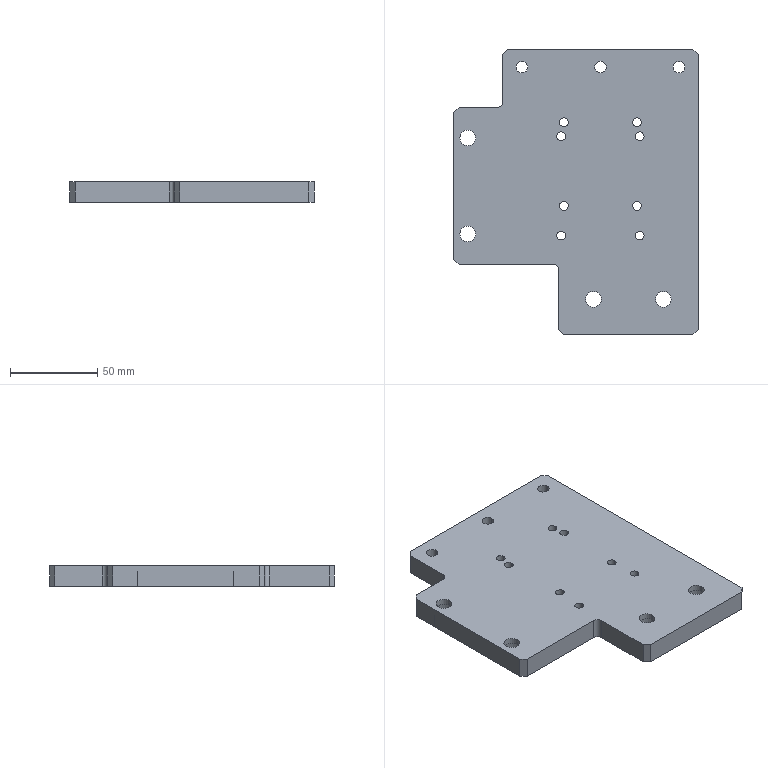Part | SolidWorks | features HoleWzd 5, Chamfer 3, Fillet 2, ICE 2, Extrusion 1, LPattern 1, MirrorPattern 1 | 1 solid | 69 faces | box 140 x 163 x 12 mm | volume 222446 mm3 | cylinder 46 | plane 23 | commonest cylinder face diameters 5 x16 9 x8 15 x8 6.6 x6 11 x6 6 x2